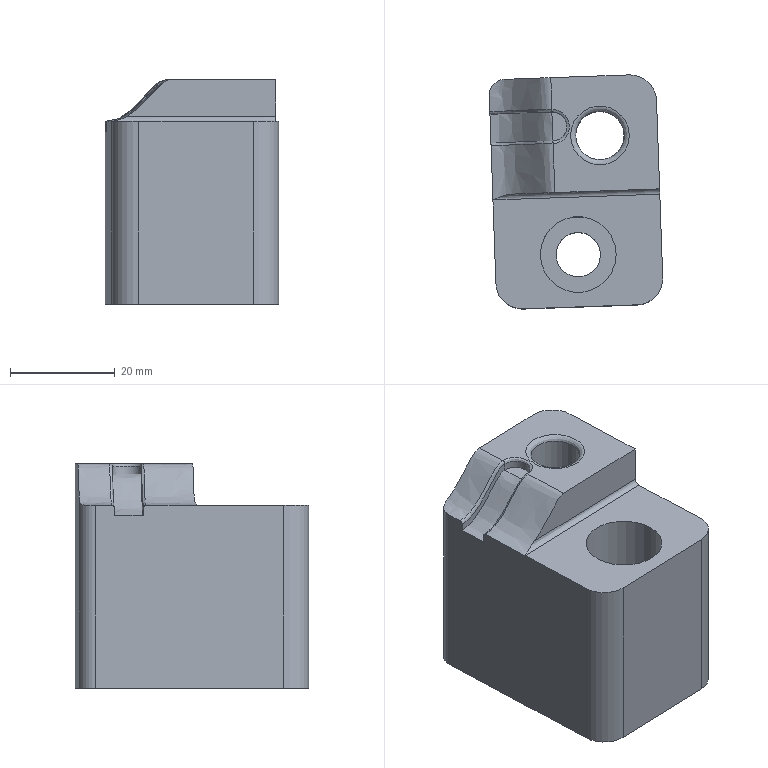Part | NX | features DIE-59 2 | 1 solid | 30 faces | box 33.188 x 44.745 x 43 mm | volume 45834 mm3 | plane 11 | cylinder 9 | spline 9 | torus 1 | commonest cylinder face diameters 10 x3 2 x1 6 x1 8.5 x1 9.27 x1 14 x1